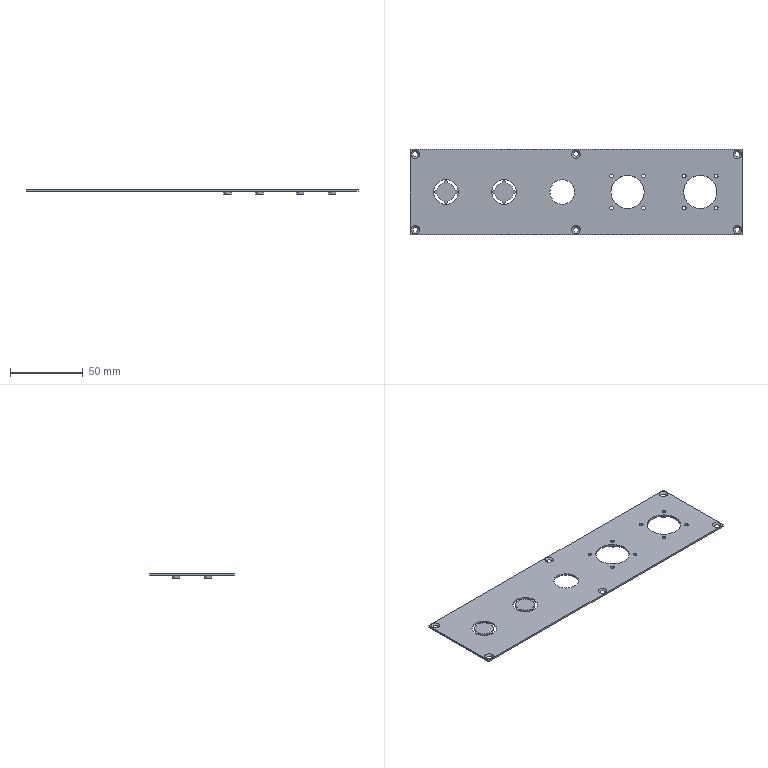Part | STEP file | FHD-021-006 rear power board | 1 solid | 79 faces | box 228.5 x 58.5 x 3.2 mm | volume 14630 mm3 | cylinder 35 | plane 30 | cone 14 | commonest cylinder face diameters 17 x9 2.5 x8 5 x8 13 x8 23 x2